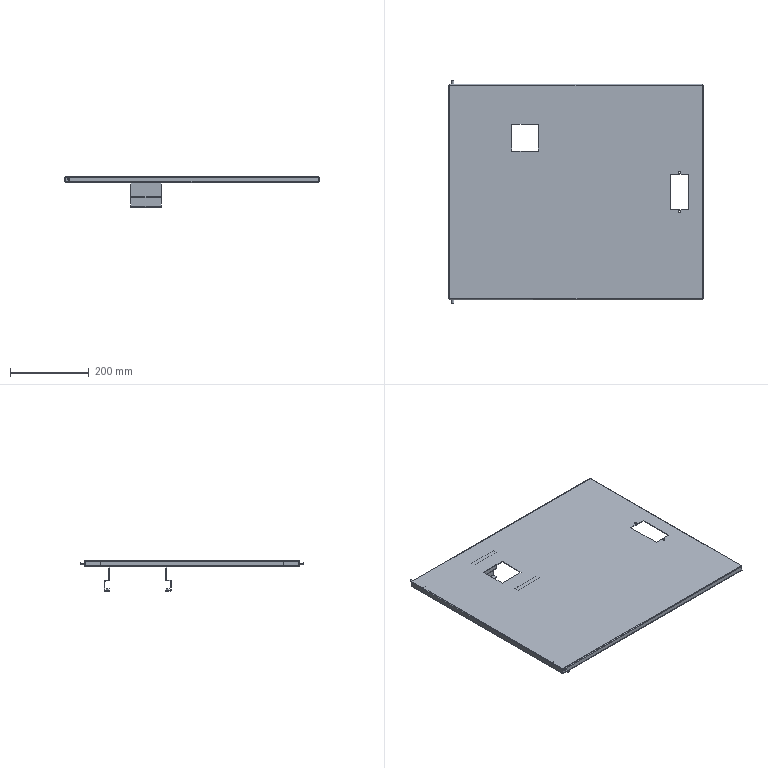Part | SolidWorks | features ICE 6, Cut 2, MirrorPattern 2, BossThin 1, Fillet 1, FlatPattern 1, Helix 1, SMBaseFlange 1, SMMiteredFlange 1, SheetMetal 1, Sweep 1, WeldmentFeature 1 | 1 solid | 178 faces | box 647 x 568 x 78 mm | volume 637931 mm3 | plane 107 | cylinder 49 | spline 22 | commonest cylinder face diameters 1.473 x9 3 x8 4.473 x8 6 x8 4 x4 4.5 x4